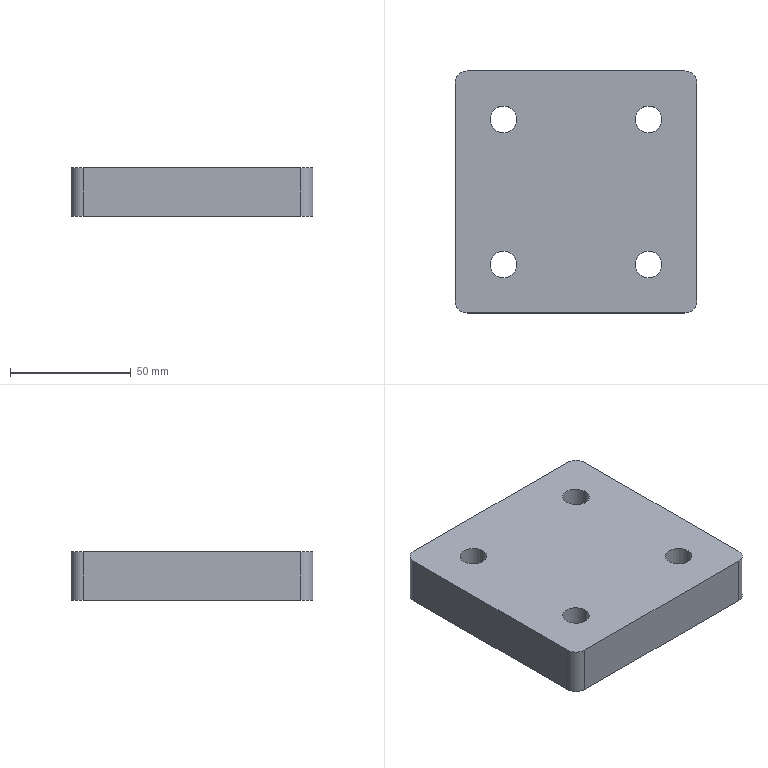Part | SolidWorks | features BaseBody 1 | 1 solid | 18 faces | box 100 x 100 x 20 mm | volume 191968 mm3 | cylinder 12 | plane 6 | commonest cylinder face diameters 11 x8 10 x4
STEP:
#1=CARTESIAN_POINT('',(-35.5,30.,0.));
#2=VERTEX_POINT('',#1);
#3=CARTESIAN_POINT('',(-24.5,30.,0.));
#4=VERTEX_POINT('',#3);
#5=CARTESIAN_POINT('',(-30.,30.,0.));
#6=DIRECTION('',(0.,0.,1.));
#7=DIRECTION('',(-1.,0.,0.));
#8=AXIS2_PLACEMENT_3D('',#5,#6,#7);
#9=CIRCLE('',#8,5.5);
#10=EDGE_CURVE('',#2,#4,#9,.T.);
#11=ORIENTED_EDGE('',*,*,#10,.F.);
#12=CARTESIAN_POINT('',(-35.5,30.,20.));
#13=VERTEX_POINT('',#12);
#14=CARTESIAN_POINT('',(-35.5,30.,0.));
#15=DIRECTION('',(0.,0.,1.));
#16=VECTOR('',#15,1000.);
#17=LINE('',#14,#16);
#18=EDGE_CURVE('',#2,#13,#17,.T.);
#19=ORIENTED_EDGE('',*,*,#18,.T.);
#20=CARTESIAN_POINT('',(-24.5,30.,20.));
#21=VERTEX_POINT('',#20);
#22=CARTESIAN_POINT('',(-30.,30.,20.));
#23=DIRECTION('',(0.,0.,1.));
#24=DIRECTION('',(-1.,0.,0.));
#25=AXIS2_PLACEMENT_3D('',#22,#23,#24);
#26=CIRCLE('',#25,5.5);
#27=EDGE_CURVE('',#13,#21,#26,.T.);
#28=ORIENTED_EDGE('',*,*,#27,.T.);
#29=CARTESIAN_POINT('',(-24.5,30.,0.));
#30=DIRECTION('',(0.,0.,1.));
#31=VECTOR('',#30,1000.);
#32=LINE('',#29,#31);
#33=EDGE_CURVE('',#4,#21,#32,.T.);
#34=ORIENTED_EDGE('',*,*,#33,.F.);
#35=EDGE_LOOP('',(#11,#19,#28,#34));
#36=FACE_OUTER_BOUND('',#35,.T.);
#37=CARTESIAN_POINT('',(-30.,30.,0.));
#38=DIRECTION('',(0.,0.,1.));
#39=DIRECTION('',(1.,0.,0.));
#40=AXIS2_PLACEMENT_3D('',#37,#38,#39);
#41=CYLINDRICAL_SURFACE('',#40,5.5);
#42=ADVANCED_FACE('',(#36),#41,.F.);
#43=CARTESIAN_POINT('',(24.5,-30.,0.));
#44=VERTEX_POINT('',#43);
#45=CARTESIAN_POINT('',(35.5,-30.,0.));
#46=VERTEX_POINT('',#45);
#47=CARTESIAN_POINT('',(30.,-30.,0.));
#48=DIRECTION('',(0.,0.,1.));
#49=DIRECTION('',(-1.,0.,0.));
#50=AXIS2_PLACEMENT_3D('',#47,#48,#49);
#51=CIRCLE('',#50,5.5);
#52=EDGE_CURVE('',#44,#46,#51,.T.);
#53=ORIENTED_EDGE('',*,*,#52,.F.);
#54=CARTESIAN_POINT('',(24.5,-30.,20.));
#55=VERTEX_POINT('',#54);
#56=CARTESIAN_POINT('',(24.5,-30.,0.));
#57=DIRECTION('',(0.,0.,1.));
#58=VECTOR('',#57,1000.);
#59=LINE('',#56,#58);
#60=EDGE_CURVE('',#44,#55,#59,.T.);
#61=ORIENTED_EDGE('',*,*,#60,.T.);
#62=CARTESIAN_POINT('',(35.5,-30.,20.));
#63=VERTEX_POINT('',#62);
#64=CARTESIAN_POINT('',(30.,-30.,20.));
#65=DIRECTION('',(0.,0.,1.));
#66=DIRECTION('',(-1.,0.,0.));
#67=AXIS2_PLACEMENT_3D('',#64,#65,#66);
#68=CIRCLE('',#67,5.5);
#69=EDGE_CURVE('',#55,#63,#68,.T.);
#70=ORIENTED_EDGE('',*,*,#69,.T.);
#71=CARTESIAN_POINT('',(35.5,-30.,0.));
#72=DIRECTION('',(0.,0.,1.));
#73=VECTOR('',#72,1000.);
#74=LINE('',#71,#73);
#75=EDGE_CURVE('',#46,#63,#74,.T.);
#76=ORIENTED_EDGE('',*,*,#75,.F.);
#77=EDGE_LOOP('',(#53,#61,#70,#76));
#78=FACE_OUTER_BOUND('',#77,.T.);
#79=CARTESIAN_POINT('',(30.,-30.,0.));
#80=DIRECTION('',(0.,0.,1.));
#81=DIRECTION('',(1.,0.,0.));
#82=AXIS2_PLACEMENT_3D('',#79,#80,#81);
#83=CYLINDRICAL_SURFACE('',#82,5.5);
#84=ADVANCED_FACE('',(#78),#83,.F.);
#85=CARTESIAN_POINT('',(24.5,30.,0.));
#86=VERTEX_POINT('',#85);
#87=CARTESIAN_POINT('',(35.5,30.,0.));
#88=VERTEX_POINT('',#87);
#89=CARTESIAN_POINT('',(30.,30.,0.));
#90=DIRECTION('',(0.,0.,1.));
#91=DIRECTION('',(1.,0.,0.));
#92=AXIS2_PLACEMENT_3D('',#89,#90,#91);
#93=CIRCLE('',#92,5.5);
#94=EDGE_CURVE('',#86,#88,#93,.T.);
#95=ORIENTED_EDGE('',*,*,#94,.F.);
#96=CARTESIAN_POINT('',(24.5,30.,20.));
#97=VERTEX_POINT('',#96);
#98=CARTESIAN_POINT('',(24.5,30.,0.));
#99=DIRECTION('',(0.,0.,1.));
#100=VECTOR('',#99,1000.);
#101=LINE('',#98,#100);
#102=EDGE_CURVE('',#86,#97,#101,.T.);
#103=ORIENTED_EDGE('',*,*,#102,.T.);
#104=CARTESIAN_POINT('',(35.5,30.,20.));
#105=VERTEX_POINT('',#104);
#106=CARTESIAN_POINT('',(30.,30.,20.));
#107=DIRECTION('',(0.,0.,1.));
#108=DIRECTION('',(1.,0.,0.));
#109=AXIS2_PLACEMENT_3D('',#106,#107,#108);
#110=CIRCLE('',#109,5.5);
#111=EDGE_CURVE('',#97,#105,#110,.T.);
#112=ORIENTED_EDGE('',*,*,#111,.T.);
#113=CARTESIAN_POINT('',(35.5,30.,0.));
#114=DIRECTION('',(0.,0.,1.));
#115=VECTOR('',#114,1000.);
#116=LINE('',#113,#115);
#117=EDGE_CURVE('',#88,#105,#116,.T.);
#118=ORIENTED_EDGE('',*,*,#117,.F.);
#119=EDGE_LOOP('',(#95,#103,#112,#118));
#120=FACE_OUTER_BOUND('',#119,.T.);
#121=CARTESIAN_POINT('',(30.,30.,0.));
#122=DIRECTION('',(0.,0.,1.));
#123=DIRECTION('',(1.,0.,0.));
#124=AXIS2_PLACEMENT_3D('',#121,#122,#123);
#125=CYLINDRICAL_SURFACE('',#124,5.5);
#126=ADVANCED_FACE('',(#120),#125,.F.);
#127=CARTESIAN_POINT('',(-35.5,-30.,0.));
#128=VERTEX_POINT('',#127);
#129=CARTESIAN_POINT('',(-24.5,-30.,0.));
#130=VERTEX_POINT('',#129);
#131=CARTESIAN_POINT('',(-30.,-30.,0.));
#132=DIRECTION('',(0.,0.,1.));
#133=DIRECTION('',(1.,0.,0.));
#134=AXIS2_PLACEMENT_3D('',#131,#132,#133);
#135=CIRCLE('',#134,5.5);
#136=EDGE_CURVE('',#128,#130,#135,.T.);
#137=ORIENTED_EDGE('',*,*,#136,.F.);
#138=CARTESIAN_POINT('',(-35.5,-30.,20.));
#139=VERTEX_POINT('',#138);
#140=CARTESIAN_POINT('',(-35.5,-30.,0.));
#141=DIRECTION('',(0.,0.,1.));
#142=VECTOR('',#141,1000.);
#143=LINE('',#140,#142);
#144=EDGE_CURVE('',#128,#139,#143,.T.);
#145=ORIENTED_EDGE('',*,*,#144,.T.);
#146=CARTESIAN_POINT('',(-24.5,-30.,20.));
#147=VERTEX_POINT('',#146);
#148=CARTESIAN_POINT('',(-30.,-30.,20.));
#149=DIRECTION('',(0.,0.,1.));
#150=DIRECTION('',(1.,0.,0.));
#151=AXIS2_PLACEMENT_3D('',#148,#149,#150);
#152=CIRCLE('',#151,5.5);
#153=EDGE_CURVE('',#139,#147,#152,.T.);
#154=ORIENTED_EDGE('',*,*,#153,.T.);
#155=CARTESIAN_POINT('',(-24.5,-30.,0.));
#156=DIRECTION('',(0.,0.,1.));
#157=VECTOR('',#156,1000.);
#158=LINE('',#155,#157);
#159=EDGE_CURVE('',#130,#147,#158,.T.);
#160=ORIENTED_EDGE('',*,*,#159,.F.);
#161=EDGE_LOOP('',(#137,#145,#154,#160));
#162=FACE_OUTER_BOUND('',#161,.T.);
#163=CARTESIAN_POINT('',(-30.,-30.,0.));
#164=DIRECTION('',(0.,0.,1.));
#165=DIRECTION('',(1.,0.,0.));
#166=AXIS2_PLACEMENT_3D('',#163,#164,#165);
#167=CYLINDRICAL_SURFACE('',#166,5.5);
#168=ADVANCED_FACE('',(#162),#167,.F.);
#169=CARTESIAN_POINT('',(50.,-45.,0.));
#170=VERTEX_POINT('',#169);
#171=CARTESIAN_POINT('',(50.,45.,0.));
#172=VERTEX_POINT('',#171);
#173=CARTESIAN_POINT('',(50.,50.,0.));
#174=DIRECTION('',(0.,1.,0.));
#175=VECTOR('',#174,1000.);
#176=LINE('',#173,#175);
#177=EDGE_CURVE('',#170,#172,#176,.T.);
#178=ORIENTED_EDGE('',*,*,#177,.T.);
#179=CARTESIAN_POINT('',(50.,45.,20.));
#180=VERTEX_POINT('',#179);
#181=CARTESIAN_POINT('',(50.,45.,20.));
#182=DIRECTION('',(0.,0.,1.));
#183=VECTOR('',#182,1000.);
#184=LINE('',#181,#183);
#185=EDGE_CURVE('',#172,#180,#184,.T.);
#186=ORIENTED_EDGE('',*,*,#185,.T.);
#187=CARTESIAN_POINT('',(50.,-45.,20.));
#188=VERTEX_POINT('',#187);
#189=CARTESIAN_POINT('',(50.,50.,20.));
#190=DIRECTION('',(0.,1.,0.));
#191=VECTOR('',#190,1000.);
#192=LINE('',#189,#191);
#193=EDGE_CURVE('',#188,#180,#192,.T.);
#194=ORIENTED_EDGE('',*,*,#193,.F.);
#195=CARTESIAN_POINT('',(50.,-45.,20.));
#196=DIRECTION('',(0.,0.,-1.));
#197=VECTOR('',#196,1000.);
#198=LINE('',#195,#197);
#199=EDGE_CURVE('',#188,#170,#198,.T.);
#200=ORIENTED_EDGE('',*,*,#199,.T.);
#201=EDGE_LOOP('',(#178,#186,#194,#200));
#202=FACE_OUTER_BOUND('',#201,.T.);
#203=CARTESIAN_POINT('',(50.,50.,20.));
#204=DIRECTION('',(-1.,0.,0.));
#205=DIRECTION('',(0.,-1.,0.));
#206=AXIS2_PLACEMENT_3D('',#203,#204,#205);
#207=PLANE('',#206);
#208=ADVANCED_FACE('',(#202),#207,.F.);
#209=CARTESIAN_POINT('',(45.,50.,0.));
#210=VERTEX_POINT('',#209);
#211=CARTESIAN_POINT('',(-45.,50.,0.));
#212=VERTEX_POINT('',#211);
#213=CARTESIAN_POINT('',(-50.,50.,0.));
#214=DIRECTION('',(-1.,0.,0.));
#215=VECTOR('',#214,1000.);
#216=LINE('',#213,#215);
#217=EDGE_CURVE('',#210,#212,#216,.T.);
#218=ORIENTED_EDGE('',*,*,#217,.T.);
#219=CARTESIAN_POINT('',(-45.,50.,20.));
#220=VERTEX_POINT('',#219);
#221=CARTESIAN_POINT('',(-45.,50.,20.));
#222=DIRECTION('',(0.,0.,1.));
#223=VECTOR('',#222,1000.);
#224=LINE('',#221,#223);
#225=EDGE_CURVE('',#212,#220,#224,.T.);
#226=ORIENTED_EDGE('',*,*,#225,.T.);
#227=CARTESIAN_POINT('',(45.,50.,20.));
#228=VERTEX_POINT('',#227);
#229=CARTESIAN_POINT('',(-50.,50.,20.));
#230=DIRECTION('',(-1.,0.,0.));
#231=VECTOR('',#230,1000.);
#232=LINE('',#229,#231);
#233=EDGE_CURVE('',#228,#220,#232,.T.);
#234=ORIENTED_EDGE('',*,*,#233,.F.);
#235=CARTESIAN_POINT('',(45.,50.,20.));
#236=DIRECTION('',(0.,0.,-1.));
#237=VECTOR('',#236,1000.);
#238=LINE('',#235,#237);
#239=EDGE_CURVE('',#228,#210,#238,.T.);
#240=ORIENTED_EDGE('',*,*,#239,.T.);
#241=EDGE_LOOP('',(#218,#226,#234,#240));
#242=FACE_OUTER_BOUND('',#241,.T.);
#243=CARTESIAN_POINT('',(-50.,50.,20.));
#244=DIRECTION('',(0.,-1.,0.));
#245=DIRECTION('',(0.,0.,-1.));
#246=AXIS2_PLACEMENT_3D('',#243,#244,#245);
#247=PLANE('',#246);
#248=ADVANCED_FACE('',(#242),#247,.F.);
#249=CARTESIAN_POINT('',(-50.,45.,0.));
#250=VERTEX_POINT('',#249);
#251=CARTESIAN_POINT('',(-50.,-45.,0.));
#252=VERTEX_POINT('',#251);
#253=CARTESIAN_POINT('',(-50.,50.,0.));
#254=DIRECTION('',(0.,-1.,0.));
#255=VECTOR('',#254,1000.);
#256=LINE('',#253,#255);
#257=EDGE_CURVE('',#250,#252,#256,.T.);
#258=ORIENTED_EDGE('',*,*,#257,.T.);
#259=CARTESIAN_POINT('',(-50.,-45.,20.));
#260=VERTEX_POINT('',#259);
#261=CARTESIAN_POINT('',(-50.,-45.,20.));
#262=DIRECTION('',(0.,0.,1.));
#263=VECTOR('',#262,1000.);
#264=LINE('',#261,#263);
#265=EDGE_CURVE('',#252,#260,#264,.T.);
#266=ORIENTED_EDGE('',*,*,#265,.T.);
#267=CARTESIAN_POINT('',(-50.,45.,20.));
#268=VERTEX_POINT('',#267);
#269=CARTESIAN_POINT('',(-50.,50.,20.));
#270=DIRECTION('',(0.,-1.,0.));
#271=VECTOR('',#270,1000.);
#272=LINE('',#269,#271);
#273=EDGE_CURVE('',#268,#260,#272,.T.);
#274=ORIENTED_EDGE('',*,*,#273,.F.);
#275=CARTESIAN_POINT('',(-50.,45.,20.));
#276=DIRECTION('',(0.,0.,-1.));
#277=VECTOR('',#276,1000.);
#278=LINE('',#275,#277);
#279=EDGE_CURVE('',#268,#250,#278,.T.);
#280=ORIENTED_EDGE('',*,*,#279,.T.);
#281=EDGE_LOOP('',(#258,#266,#274,#280));
#282=FACE_OUTER_BOUND('',#281,.T.);
#283=CARTESIAN_POINT('',(-50.,50.,20.));
#284=DIRECTION('',(1.,0.,0.));
#285=DIRECTION('',(0.,1.,0.));
#286=AXIS2_PLACEMENT_3D('',#283,#284,#285);
#287=PLANE('',#286);
#288=ADVANCED_FACE('',(#282),#287,.F.);
#289=CARTESIAN_POINT('',(-45.,-50.,20.));
#290=VERTEX_POINT('',#289);
#291=CARTESIAN_POINT('',(45.,-50.,20.));
#292=VERTEX_POINT('',#291);
#293=CARTESIAN_POINT('',(-50.,-50.,20.));
#294=DIRECTION('',(1.,0.,0.));
#295=VECTOR('',#294,1000.);
#296=LINE('',#293,#295);
#297=EDGE_CURVE('',#290,#292,#296,.T.);
#298=ORIENTED_EDGE('',*,*,#297,.F.);
#299=CARTESIAN_POINT('',(-45.,-50.,0.));
#300=VERTEX_POINT('',#299);
#301=CARTESIAN_POINT('',(-45.,-50.,20.));
#302=DIRECTION('',(0.,0.,-1.));
#303=VECTOR('',#302,1000.);
#304=LINE('',#301,#303);
#305=EDGE_CURVE('',#290,#300,#304,.T.);
#306=ORIENTED_EDGE('',*,*,#305,.T.);
#307=CARTESIAN_POINT('',(45.,-50.,0.));
#308=VERTEX_POINT('',#307);
#309=CARTESIAN_POINT('',(-50.,-50.,0.));
#310=DIRECTION('',(1.,0.,0.));
#311=VECTOR('',#310,1000.);
#312=LINE('',#309,#311);
#313=EDGE_CURVE('',#300,#308,#312,.T.);
#314=ORIENTED_EDGE('',*,*,#313,.T.);
#315=CARTESIAN_POINT('',(45.,-50.,20.));
#316=DIRECTION('',(0.,0.,1.));
#317=VECTOR('',#316,1000.);
#318=LINE('',#315,#317);
#319=EDGE_CURVE('',#308,#292,#318,.T.);
#320=ORIENTED_EDGE('',*,*,#319,.T.);
#321=EDGE_LOOP('',(#298,#306,#314,#320));
#322=FACE_OUTER_BOUND('',#321,.T.);
#323=CARTESIAN_POINT('',(-50.,-50.,20.));
#324=DIRECTION('',(0.,1.,0.));
#325=DIRECTION('',(0.,0.,1.));
#326=AXIS2_PLACEMENT_3D('',#323,#324,#325);
#327=PLANE('',#326);
#328=ADVANCED_FACE('',(#322),#327,.F.);
#329=CARTESIAN_POINT('',(-30.,30.,20.));
#330=DIRECTION('',(0.,0.,1.));
#331=DIRECTION('',(-1.,0.,0.));
#332=AXIS2_PLACEMENT_3D('',#329,#330,#331);
#333=CIRCLE('',#332,5.5);
#334=EDGE_CURVE('',#21,#13,#333,.T.);
#335=ORIENTED_EDGE('',*,*,#334,.F.);
#336=ORIENTED_EDGE('',*,*,#27,.F.);
#337=EDGE_LOOP('',(#335,#336));
#338=FACE_BOUND('',#337,.T.);
#339=CARTESIAN_POINT('',(30.,-30.,20.));
#340=DIRECTION('',(0.,0.,1.));
#341=DIRECTION('',(-1.,0.,0.));
#342=AXIS2_PLACEMENT_3D('',#339,#340,#341);
#343=CIRCLE('',#342,5.5);
#344=EDGE_CURVE('',#63,#55,#343,.T.);
#345=ORIENTED_EDGE('',*,*,#344,.F.);
#346=ORIENTED_EDGE('',*,*,#69,.F.);
#347=EDGE_LOOP('',(#345,#346));
#348=FACE_BOUND('',#347,.T.);
#349=CARTESIAN_POINT('',(30.,30.,20.));
#350=DIRECTION('',(0.,0.,1.));
#351=DIRECTION('',(1.,0.,0.));
#352=AXIS2_PLACEMENT_3D('',#349,#350,#351);
#353=CIRCLE('',#352,5.5);
#354=EDGE_CURVE('',#105,#97,#353,.T.);
#355=ORIENTED_EDGE('',*,*,#354,.F.);
#356=ORIENTED_EDGE('',*,*,#111,.F.);
#357=EDGE_LOOP('',(#355,#356));
#358=FACE_BOUND('',#357,.T.);
#359=CARTESIAN_POINT('',(-30.,-30.,20.));
#360=DIRECTION('',(0.,0.,1.));
#361=DIRECTION('',(1.,0.,0.));
#362=AXIS2_PLACEMENT_3D('',#359,#360,#361);
#363=CIRCLE('',#362,5.5);
#364=EDGE_CURVE('',#147,#139,#363,.T.);
#365=ORIENTED_EDGE('',*,*,#364,.F.);
#366=ORIENTED_EDGE('',*,*,#153,.F.);
#367=EDGE_LOOP('',(#365,#366));
#368=FACE_BOUND('',#367,.T.);
#369=ORIENTED_EDGE('',*,*,#273,.T.);
#370=CARTESIAN_POINT('',(-45.,-45.,20.));
#371=DIRECTION('',(0.,0.,1.));
#372=DIRECTION('',(1.,0.,0.));
#373=AXIS2_PLACEMENT_3D('',#370,#371,#372);
#374=CIRCLE('',#373,5.);
#375=EDGE_CURVE('',#260,#290,#374,.T.);
#376=ORIENTED_EDGE('',*,*,#375,.T.);
#377=ORIENTED_EDGE('',*,*,#297,.T.);
#378=CARTESIAN_POINT('',(45.,-45.,20.));
#379=DIRECTION('',(0.,0.,1.));
#380=DIRECTION('',(1.,0.,0.));
#381=AXIS2_PLACEMENT_3D('',#378,#379,#380);
#382=CIRCLE('',#381,5.);
#383=EDGE_CURVE('',#292,#188,#382,.T.);
#384=ORIENTED_EDGE('',*,*,#383,.T.);
#385=ORIENTED_EDGE('',*,*,#193,.T.);
#386=CARTESIAN_POINT('',(45.,45.,20.));
#387=DIRECTION('',(0.,0.,1.));
#388=DIRECTION('',(1.,0.,0.));
#389=AXIS2_PLACEMENT_3D('',#386,#387,#388);
#390=CIRCLE('',#389,5.);
#391=EDGE_CURVE('',#180,#228,#390,.T.);
#392=ORIENTED_EDGE('',*,*,#391,.T.);
#393=ORIENTED_EDGE('',*,*,#233,.T.);
#394=CARTESIAN_POINT('',(-45.,45.,20.));
#395=DIRECTION('',(0.,0.,1.));
#396=DIRECTION('',(1.,0.,0.));
#397=AXIS2_PLACEMENT_3D('',#394,#395,#396);
#398=CIRCLE('',#397,5.);
#399=EDGE_CURVE('',#220,#268,#398,.T.);
#400=ORIENTED_EDGE('',*,*,#399,.T.);
#401=EDGE_LOOP('',(#369,#376,#377,#384,#385,#392,#393,#400));
#402=FACE_OUTER_BOUND('',#401,.T.);
#403=CARTESIAN_POINT('',(0.,0.,20.));
#404=DIRECTION('',(0.,0.,1.));
#405=DIRECTION('',(1.,0.,0.));
#406=AXIS2_PLACEMENT_3D('',#403,#404,#405);
#407=PLANE('',#406);
#408=ADVANCED_FACE('',(#338,#348,#358,#368,#402),#407,.T.);
#409=CARTESIAN_POINT('',(-30.,30.,0.));
#410=DIRECTION('',(0.,0.,1.));
#411=DIRECTION('',(-1.,0.,0.));
#412=AXIS2_PLACEMENT_3D('',#409,#410,#411);
#413=CIRCLE('',#412,5.5);
#414=EDGE_CURVE('',#4,#2,#413,.T.);
#415=ORIENTED_EDGE('',*,*,#414,.T.);
#416=ORIENTED_EDGE('',*,*,#10,.T.);
#417=EDGE_LOOP('',(#415,#416));
#418=FACE_BOUND('',#417,.T.);
#419=CARTESIAN_POINT('',(30.,-30.,0.));
#420=DIRECTION('',(0.,0.,1.));
#421=DIRECTION('',(-1.,0.,0.));
#422=AXIS2_PLACEMENT_3D('',#419,#420,#421);
#423=CIRCLE('',#422,5.5);
#424=EDGE_CURVE('',#46,#44,#423,.T.);
#425=ORIENTED_EDGE('',*,*,#424,.T.);
#426=ORIENTED_EDGE('',*,*,#52,.T.);
#427=EDGE_LOOP('',(#425,#426));
#428=FACE_BOUND('',#427,.T.);
#429=CARTESIAN_POINT('',(30.,30.,0.));
#430=DIRECTION('',(0.,0.,1.));
#431=DIRECTION('',(1.,0.,0.));
#432=AXIS2_PLACEMENT_3D('',#429,#430,#431);
#433=CIRCLE('',#432,5.5);
#434=EDGE_CURVE('',#88,#86,#433,.T.);
#435=ORIENTED_EDGE('',*,*,#434,.T.);
#436=ORIENTED_EDGE('',*,*,#94,.T.);
#437=EDGE_LOOP('',(#435,#436));
#438=FACE_BOUND('',#437,.T.);
#439=CARTESIAN_POINT('',(-30.,-30.,0.));
#440=DIRECTION('',(0.,0.,1.));
#441=DIRECTION('',(1.,0.,0.));
#442=AXIS2_PLACEMENT_3D('',#439,#440,#441);
#443=CIRCLE('',#442,5.5);
#444=EDGE_CURVE('',#130,#128,#443,.T.);
#445=ORIENTED_EDGE('',*,*,#444,.T.);
#446=ORIENTED_EDGE('',*,*,#136,.T.);
#447=EDGE_LOOP('',(#445,#446));
#448=FACE_BOUND('',#447,.T.);
#449=ORIENTED_EDGE('',*,*,#313,.F.);
#450=CARTESIAN_POINT('',(-45.,-45.,0.));
#451=DIRECTION('',(0.,0.,-1.));
#452=DIRECTION('',(1.,0.,0.));
#453=AXIS2_PLACEMENT_3D('',#450,#451,#452);
#454=CIRCLE('',#453,5.);
#455=EDGE_CURVE('',#300,#252,#454,.T.);
#456=ORIENTED_EDGE('',*,*,#455,.T.);
#457=ORIENTED_EDGE('',*,*,#257,.F.);
#458=CARTESIAN_POINT('',(-45.,45.,0.));
#459=DIRECTION('',(0.,0.,-1.));
#460=DIRECTION('',(1.,0.,0.));
#461=AXIS2_PLACEMENT_3D('',#458,#459,#460);
#462=CIRCLE('',#461,5.);
#463=EDGE_CURVE('',#250,#212,#462,.T.);
#464=ORIENTED_EDGE('',*,*,#463,.T.);
#465=ORIENTED_EDGE('',*,*,#217,.F.);
#466=CARTESIAN_POINT('',(45.,45.,0.));
#467=DIRECTION('',(0.,0.,-1.));
#468=DIRECTION('',(1.,0.,0.));
#469=AXIS2_PLACEMENT_3D('',#466,#467,#468);
#470=CIRCLE('',#469,5.);
#471=EDGE_CURVE('',#210,#172,#470,.T.);
#472=ORIENTED_EDGE('',*,*,#471,.T.);
#473=ORIENTED_EDGE('',*,*,#177,.F.);
#474=CARTESIAN_POINT('',(45.,-45.,0.));
#475=DIRECTION('',(0.,0.,-1.));
#476=DIRECTION('',(1.,0.,0.));
#477=AXIS2_PLACEMENT_3D('',#474,#475,#476);
#478=CIRCLE('',#477,5.);
#479=EDGE_CURVE('',#170,#308,#478,.T.);
#480=ORIENTED_EDGE('',*,*,#479,.T.);
#481=EDGE_LOOP('',(#449,#456,#457,#464,#465,#472,#473,#480));
#482=FACE_OUTER_BOUND('',#481,.T.);
#483=CARTESIAN_POINT('',(0.,0.,0.));
#484=DIRECTION('',(0.,0.,1.));
#485=DIRECTION('',(1.,0.,0.));
#486=AXIS2_PLACEMENT_3D('',#483,#484,#485);
#487=PLANE('',#486);
#488=ADVANCED_FACE('',(#418,#428,#438,#448,#482),#487,.F.);
#489=ORIENTED_EDGE('',*,*,#144,.F.);
#490=ORIENTED_EDGE('',*,*,#444,.F.);
#491=ORIENTED_EDGE('',*,*,#159,.T.);
#492=ORIENTED_EDGE('',*,*,#364,.T.);
#493=EDGE_LOOP('',(#489,#490,#491,#492));
#494=FACE_OUTER_BOUND('',#493,.T.);
#495=CARTESIAN_POINT('',(-30.,-30.,0.));
#496=DIRECTION('',(0.,0.,1.));
#497=DIRECTION('',(1.,0.,0.));
#498=AXIS2_PLACEMENT_3D('',#495,#496,#497);
#499=CYLINDRICAL_SURFACE('',#498,5.5);
#500=ADVANCED_FACE('',(#494),#499,.F.);
#501=ORIENTED_EDGE('',*,*,#102,.F.);
#502=ORIENTED_EDGE('',*,*,#434,.F.);
#503=ORIENTED_EDGE('',*,*,#117,.T.);
#504=ORIENTED_EDGE('',*,*,#354,.T.);
#505=EDGE_LOOP('',(#501,#502,#503,#504));
#506=FACE_OUTER_BOUND('',#505,.T.);
#507=CARTESIAN_POINT('',(30.,30.,0.));
#508=DIRECTION('',(0.,0.,1.));
#509=DIRECTION('',(1.,0.,0.));
#510=AXIS2_PLACEMENT_3D('',#507,#508,#509);
#511=CYLINDRICAL_SURFACE('',#510,5.5);
#512=ADVANCED_FACE('',(#506),#511,.F.);
#513=ORIENTED_EDGE('',*,*,#60,.F.);
#514=ORIENTED_EDGE('',*,*,#424,.F.);
#515=ORIENTED_EDGE('',*,*,#75,.T.);
#516=ORIENTED_EDGE('',*,*,#344,.T.);
#517=EDGE_LOOP('',(#513,#514,#515,#516));
#518=FACE_OUTER_BOUND('',#517,.T.);
#519=CARTESIAN_POINT('',(30.,-30.,0.));
#520=DIRECTION('',(0.,0.,1.));
#521=DIRECTION('',(1.,0.,0.));
#522=AXIS2_PLACEMENT_3D('',#519,#520,#521);
#523=CYLINDRICAL_SURFACE('',#522,5.5);
#524=ADVANCED_FACE('',(#518),#523,.F.);
#525=ORIENTED_EDGE('',*,*,#18,.F.);
#526=ORIENTED_EDGE('',*,*,#414,.F.);
#527=ORIENTED_EDGE('',*,*,#33,.T.);
#528=ORIENTED_EDGE('',*,*,#334,.T.);
#529=EDGE_LOOP('',(#525,#526,#527,#528));
#530=FACE_OUTER_BOUND('',#529,.T.);
#531=CARTESIAN_POINT('',(-30.,30.,0.));
#532=DIRECTION('',(0.,0.,1.));
#533=DIRECTION('',(1.,0.,0.));
#534=AXIS2_PLACEMENT_3D('',#531,#532,#533);
#535=CYLINDRICAL_SURFACE('',#534,5.5);
#536=ADVANCED_FACE('',(#530),#535,.F.);
#537=ORIENTED_EDGE('',*,*,#375,.F.);
#538=ORIENTED_EDGE('',*,*,#265,.F.);
#539=ORIENTED_EDGE('',*,*,#455,.F.);
#540=ORIENTED_EDGE('',*,*,#305,.F.);
#541=EDGE_LOOP('',(#537,#538,#539,#540));
#542=FACE_OUTER_BOUND('',#541,.T.);
#543=CARTESIAN_POINT('',(-45.,-45.,20.));
#544=DIRECTION('',(0.,0.,-1.));
#545=DIRECTION('',(-1.,0.,0.));
#546=AXIS2_PLACEMENT_3D('',#543,#544,#545);
#547=CYLINDRICAL_SURFACE('',#546,5.);
#548=ADVANCED_FACE('',(#542),#547,.T.);
#549=ORIENTED_EDGE('',*,*,#399,.F.);
#550=ORIENTED_EDGE('',*,*,#225,.F.);
#551=ORIENTED_EDGE('',*,*,#463,.F.);
#552=ORIENTED_EDGE('',*,*,#279,.F.);
#553=EDGE_LOOP('',(#549,#550,#551,#552));
#554=FACE_OUTER_BOUND('',#553,.T.);
#555=CARTESIAN_POINT('',(-45.,45.,20.));
#556=DIRECTION('',(0.,0.,-1.));
#557=DIRECTION('',(-1.,0.,0.));
#558=AXIS2_PLACEMENT_3D('',#555,#556,#557);
#559=CYLINDRICAL_SURFACE('',#558,5.);
#560=ADVANCED_FACE('',(#554),#559,.T.);
#561=ORIENTED_EDGE('',*,*,#391,.F.);
#562=ORIENTED_EDGE('',*,*,#185,.F.);
#563=ORIENTED_EDGE('',*,*,#471,.F.);
#564=ORIENTED_EDGE('',*,*,#239,.F.);
#565=EDGE_LOOP('',(#561,#562,#563,#564));
#566=FACE_OUTER_BOUND('',#565,.T.);
#567=CARTESIAN_POINT('',(45.,45.,20.));
#568=DIRECTION('',(0.,0.,-1.));
#569=DIRECTION('',(-1.,0.,0.));
#570=AXIS2_PLACEMENT_3D('',#567,#568,#569);
#571=CYLINDRICAL_SURFACE('',#570,5.);
#572=ADVANCED_FACE('',(#566),#571,.T.);
#573=ORIENTED_EDGE('',*,*,#383,.F.);
#574=ORIENTED_EDGE('',*,*,#319,.F.);
#575=ORIENTED_EDGE('',*,*,#479,.F.);
#576=ORIENTED_EDGE('',*,*,#199,.F.);
#577=EDGE_LOOP('',(#573,#574,#575,#576));
#578=FACE_OUTER_BOUND('',#577,.T.);
#579=CARTESIAN_POINT('',(45.,-45.,20.));
#580=DIRECTION('',(0.,0.,-1.));
#581=DIRECTION('',(-1.,0.,0.));
#582=AXIS2_PLACEMENT_3D('',#579,#580,#581);
#583=CYLINDRICAL_SURFACE('',#582,5.);
#584=ADVANCED_FACE('',(#578),#583,.T.);
#585=CLOSED_SHELL('',(#42,#84,#126,#168,#208,#248,#288,#328,#408,#488,#500,#512,#524,#536,#548,#560,#572,#584));
#586=MANIFOLD_SOLID_BREP('',#585);
#587=CARTESIAN_POINT('',(0.,0.,0.));
#588=DIRECTION('',(0.,0.,1.));
#589=DIRECTION('',(1.,0.,0.));
#590=AXIS2_PLACEMENT_3D('',#587,#588,#589);
#591=(LENGTH_UNIT()NAMED_UNIT(*)SI_UNIT(.MILLI.,.METRE.));
#592=UNCERTAINTY_MEASURE_WITH_UNIT(LENGTH_MEASURE(0.00001),#591,'','');
#593=(NAMED_UNIT(*)PLANE_ANGLE_UNIT()SI_UNIT($,.RADIAN.));
#594=(NAMED_UNIT(*)SI_UNIT($,.STERADIAN.)SOLID_ANGLE_UNIT());
#595=(GEOMETRIC_REPRESENTATION_CONTEXT(3)GLOBAL_UNCERTAINTY_ASSIGNED_CONTEXT((#592))GLOBAL_UNIT_ASSIGNED_CONTEXT((#591,#593,#594))REPRESENTATION_CONTEXT('',''));
#596=ADVANCED_BREP_SHAPE_REPRESENTATION('',(#586,#590),#595);